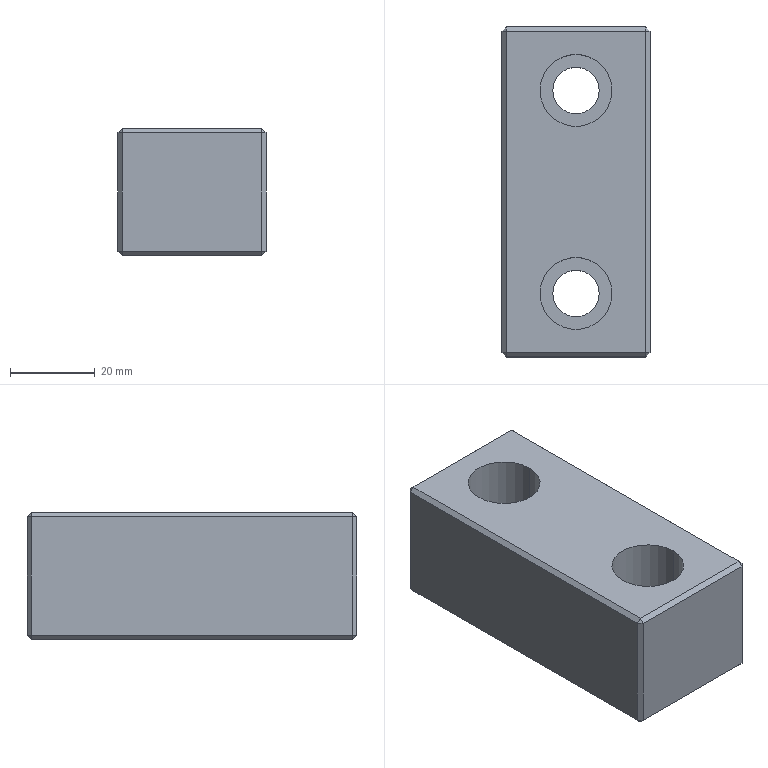Part | 1 solid | 36 faces | box 35 x 78 x 30 mm | volume 72486 mm3 | plane 28 | cylinder 8 | commonest cylinder face diameters 11 x4 17 x4